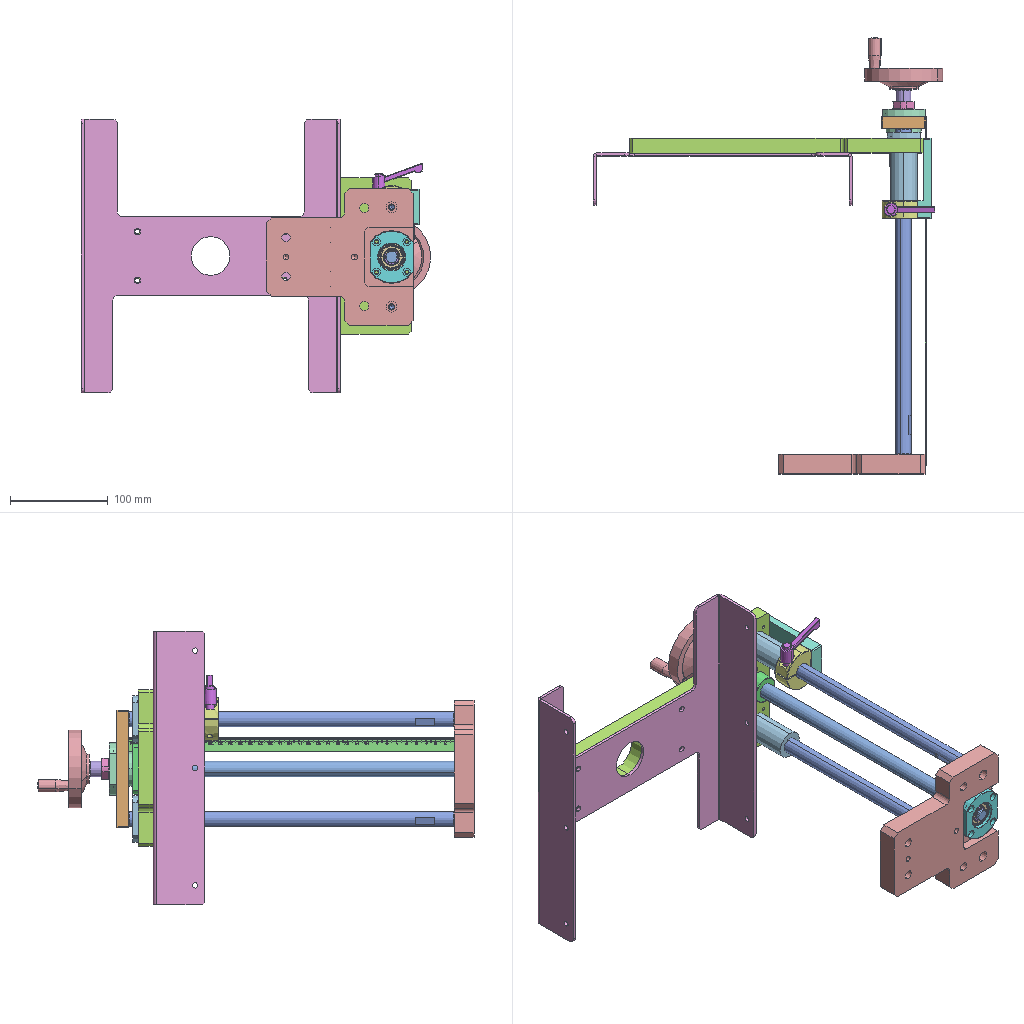Assembly | SolidWorks | 26 different items | 29 placed | box 357 x 446 x 280 mm
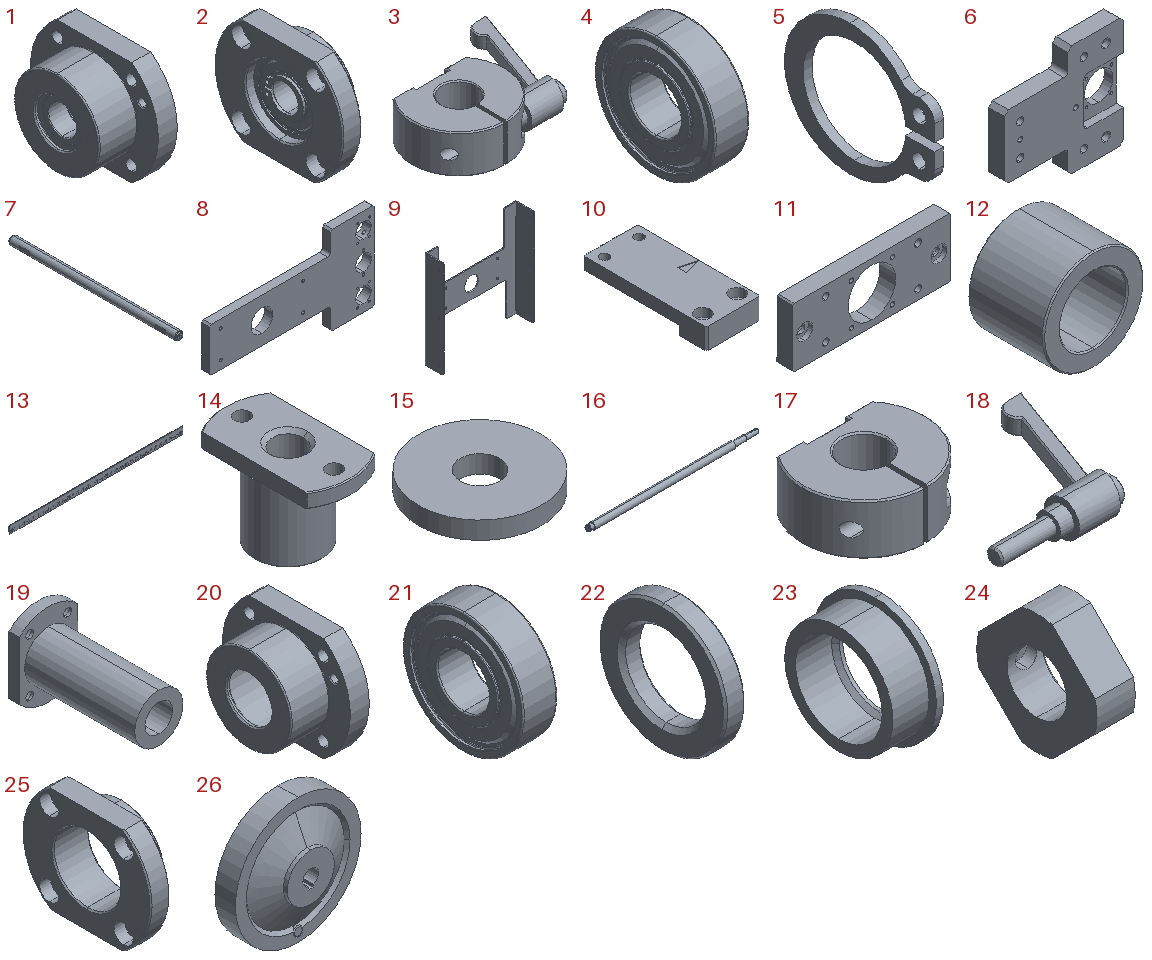Parts list (item | name | quantity | parent item | size | volume | features):
1 | (subassembly) | x1 | - | 31.5 x 54 x 44 mm | 27401 mm3 | -
2 | (subassembly) | x1 | - | 15 x 54 x 44 mm | 16597 mm3 | -
3 | (subassembly) | x1 | - | 67 x 53.987 x 18 mm | 21962 mm3 | -
4 | - | x1 | in 2 | 8 x 28 x 28 mm | 3202 mm3 | features BaseBody 1
5 | - | x1 | in 2 | 1 x 16.8 x 14.65 mm | 77.17 mm3 | features BaseBody 1
6 | - | x1 | - | 150 x 20 x 140 mm | 269906 mm3 | features HoleWzd 7, Chamfer 2, Cut 2, Fillet 2, ICE 2, Extrusion 1
7 | - | x2 | - | 16 x 339 x 16 mm | 66505 mm3 | features Chamfer 3, ICE 3, HoleWzd 2, Extrusion 1, MirrorPattern 1
8 | - | x1 | - | 300 x 15 x 160 mm | 405397 mm3 | features HoleWzd 4, ICE 3, Chamfer 2, Cut 1, Extrusion 1, Fillet 1
9 | - | x1 | - | 264.5 x 53 x 280 mm | 182601 mm3 | features HoleWzd 2, ICE 2, Fillet 1, FlatPattern 1, SMBaseFlange 1, SheetMetal 1
10 | - | x1 | - | 36 x 82 x 14 mm | 25723 mm3 | features ICE 2, Chamfer 1, Extrusion 1, HoleWzd 1
11 | - | x1 | - | 120 x 12 x 45 mm | 48954 mm3 | features HoleWzd 4, ICE 2, Chamfer 1, Extrusion 1
12 | - | x1 | - | 16 x 12 x 16 mm | 1350 mm3 | features Chamfer 1, Extrusion 1
13 | - | x1 | - | 356 x 1 x 15 mm | 5253 mm3 | features ICE 5, LPattern 3, Extrusion 1, Fillet 1
14 | - | x1 | - | 28.8 x 52 x 35 mm | 21014 mm3 | features BaseBody 1
15 | - | x1 | - | 14 x 14 x 2 mm | 276.067 mm3 | features Extrusion 1
16 | - | x1 | - | 409 x 16 x 16 mm | 74846 mm3 | features BaseBody 1
17 | - | x1 | in 3 | 44 x 35.987 x 18 mm | 17414 mm3 | features BaseBody 1
18 | - | x1 | in 3 | 55 x 51.5 x 13 mm | 4548 mm3 | features BaseBody 1
19 | - | x2 | - | 34 x 70 x 48 mm | 33217 mm3 | features ICE 3, Extrusion 1, HoleWzd 1
20 | - | x1 | in 1 | 24 x 54 x 44 mm | 16964 mm3 | features BaseBody 1
21 | - | x2 | in 1 | 8 x 28 x 28 mm | 3203 mm3 | features BaseBody 1
22 | - | x1 | in 1 | 4.8 x 30 x 30 mm | 1929 mm3 | features BaseBody 1
23 | - | x1 | in 1 | 6 x 17 x 17 mm | 446.259 mm3 | features BaseBody 1
24 | - | x1 | in 1 | 6.99 x 22 x 22 mm | 1658 mm3 | features BaseBody 1
25 | - | x1 | in 2 | 15 x 54 x 44 mm | 13318 mm3 | features BaseBody 1
26 | - | x1 | - | 80 x 52.448 x 80.5 mm | 63637 mm3 | features BaseBody 1
Mates (type | each side: item.copy, entity, surface, feature):
Coincident | 6.1 plane | assembly plane | 2 times
Concentric | 6.1 face cylinder Cut-Extrude1 | 7.1 face cylinder Boss-Extrude1
Coincident | 6.1 face plane Boss-Extrude1 | 7.1 face plane Boss-Extrude1
Concentric | 6.1 face cylinder Cut-Extrude1 | 7.2 face cylinder Boss-Extrude1
Coincident | 6.1 face plane Boss-Extrude1 | 7.2 face plane Boss-Extrude1
Concentric | 8.1 face cylinder Cut-Extrude1 | 19.1 face cylinder Boss-Extrude1
Coincident | 8.1 face plane Boss-Extrude1 | 19.1 face plane Boss-Extrude2
Concentric | 8.1 face cylinder Cut-Extrude1 | 19.2 face cylinder Boss-Extrude1
Coincident | 8.1 face plane Boss-Extrude1 | 19.2 face plane Boss-Extrude2
Concentric | 7.2 face cylinder Boss-Extrude1 | 19.2 face cylinder Boss-Extrude1
Concentric | 8.1 face cylinder M4 Tapped Hole1 | 19.1 face cylinder Hole size per socket head cap screw type1
Concentric | 8.1 face cylinder M4 Tapped Hole1 | 19.2 face cylinder Hole size per socket head cap screw type1
Concentric | 7.1 face cylinder Boss-Extrude1 | 11.1 face cylinder Hole size per socket head cap screw type1
Concentric | 7.2 face cylinder Boss-Extrude1 | 11.1 face cylinder Hole size per socket head cap screw type1
Coincident | 7.2 face plane Boss-Extrude1 | 11.1 face plane Boss-Extrude1
Concentric | 8.1 face cylinder Cut-Extrude2 | 14.1 face cylinder Input1
Concentric | 8.1 face cylinder M6 Tapped Hole1 | 14.1 face cylinder Input1
Coincident | 8.1 face plane Boss-Extrude1 | 14.1 face plane Input1
Concentric | 11.1 face cylinder Cut-Extrude1 | 20.1 face cylinder Input1
Coincident | 11.1 face plane Boss-Extrude1 | 20.1 face plane Input1
Concentric | 11.1 face cylinder M4 Tapped Hole1 | 20.1 face cylinder Input1
Coincident | 26.1 face plane Input1 | 16.1 face plane C-MTSWK16-409-S30-KE0-C16 | 2 times
Concentric | 25.1 face cylinder Input1 | 16.1 face cylinder C-MTSWK16-409-S30-KE0-C16
Concentric | 6.1 face cylinder M4 Tapped Hole1 | 25.1 face cylinder Input1
Coincident | 6.1 face plane Cut-Extrude5 | 25.1 face plane Input1
Coincident | 4.1 face plane Input1 | 16.1 face plane C-MTSWK16-409-S30-KE0-C16
Concentric | 6.1 face cylinder Cut-Extrude2 | 25.1 face cylinder Input1
Coincident | 6.1 face plane Boss-Extrude1 | 13.1 face plane Boss-Extrude1
LimitDistanceDim | 20.1 face plane Input1 | 14.1 face plane Input1
Coincident | 24.1 face plane Input1 | 12.1 face plane Boss-Extrude1
Concentric | 13.1 face cylinder Cut-Extrude4 | 6.1 face cylinder M4 Tapped Hole3
DistanceDim | 6.1 face plane Boss-Extrude1 | assembly plane
Concentric | 8.1 face cylinder M5 Tapped Hole2 | 10.1 face cylinder Cut-Extrude1
Coincident | 8.1 face plane Boss-Extrude1 | 10.1 face plane Boss-Extrude1
Concentric | 10.1 face cylinder Hole size per socket head cap screw type1 | 17.1 face cylinder Input1 | 2 times
Concentric | 7.1 face cylinder Boss-Extrude1 | 17.1 face cylinder Input1
Concentric | 26.1 face cylinder Input1 | 16.1 face cylinder C-MTSWK16-409-S30-KE0-C16
Concentric | 26.1 face cylinder Input1 | 15.1 face cylinder Boss-Extrude1
Coincident | 26.1 face plane Input1 | 15.1 face plane Boss-Extrude1
Concentric | 14.1 face cylinder Input1 | 16.1 face cylinder C-MTSWK16-409-S30-KE0-C16
Concentric | 8.1 face cylinder M6 Tapped Hole2 | 9.1 face cylinder M6 Clearance Hole1 | 2 times
Coincident | 8.1 face plane Boss-Extrude1 | 9.1 face plane Base-Flange1
Concentric | 12.1 face cylinder Boss-Extrude1 | 16.1 face cylinder C-MTSWK16-409-S30-KE0-C16
Coincident | 6.1 face plane Cut-Extrude5 | 13.1 face plane Boss-Extrude1